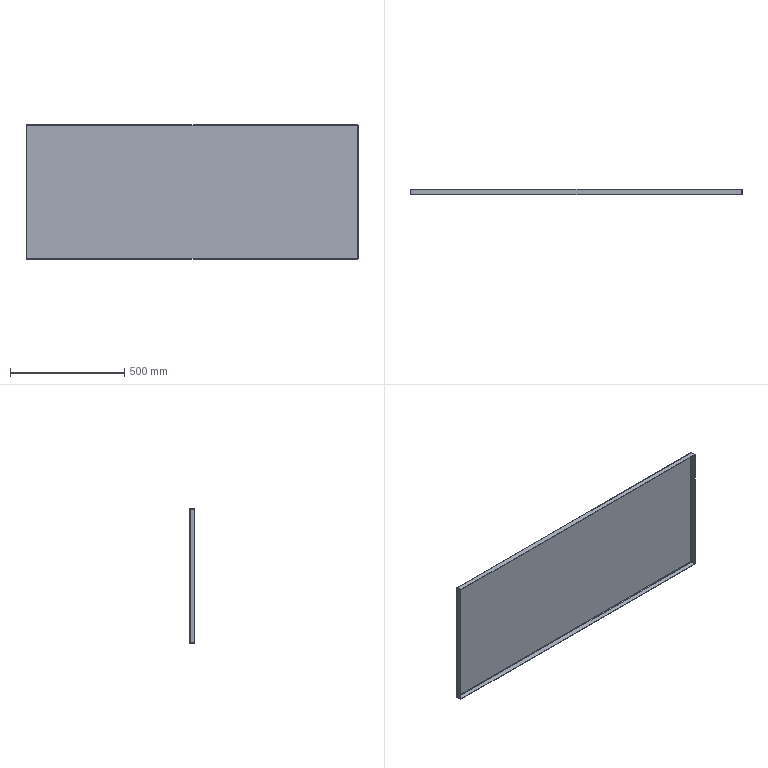Part | SolidWorks | features EdgeFlange 1, FlatPattern 1, SMBaseFlange 1, SheetMetal 1 | 1 solid | 38 faces | box 1456 x 25 x 590 mm | volume 1894739 mm3 | plane 22 | spline 8 | cylinder 8 | commonest cylinder face diameters 4 x4 8 x4